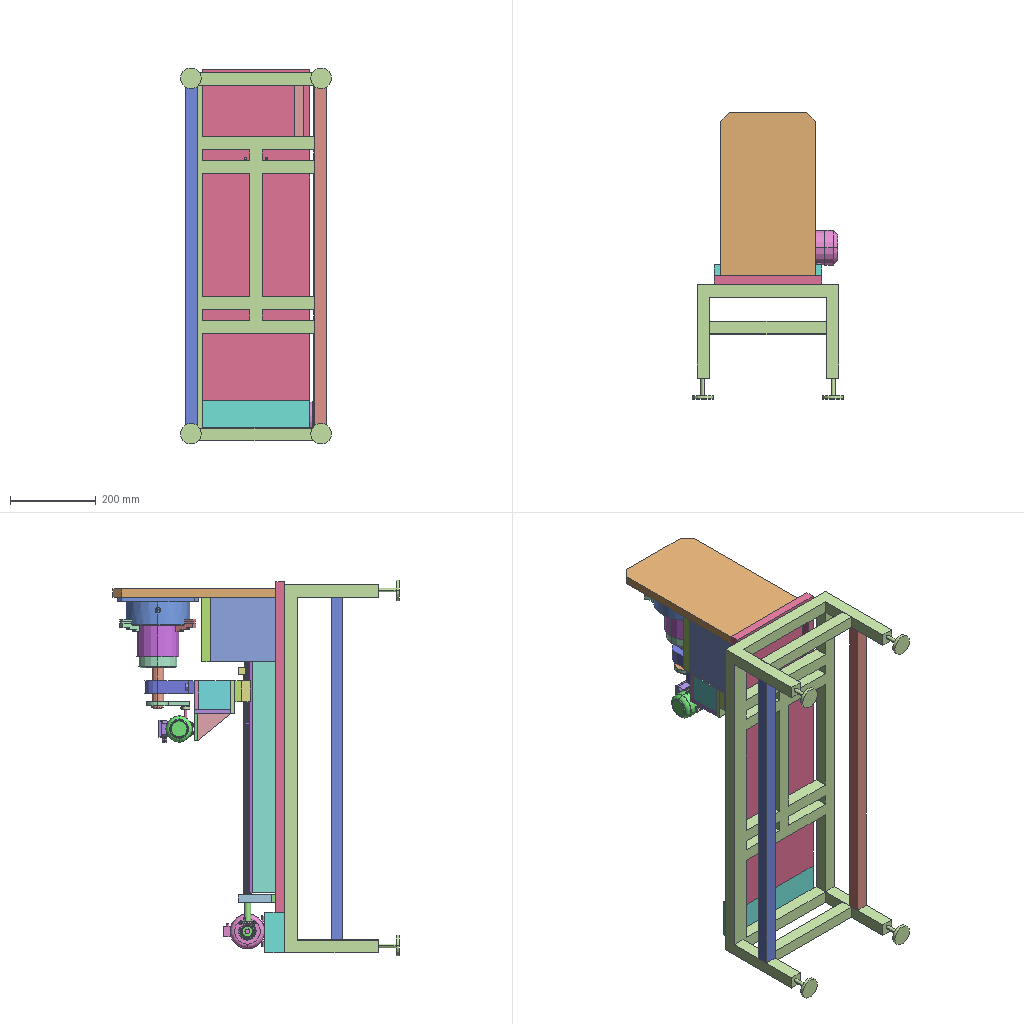Assembly | SolidWorks | 35 different items | 78 placed | box 352 x 667 x 876 mm
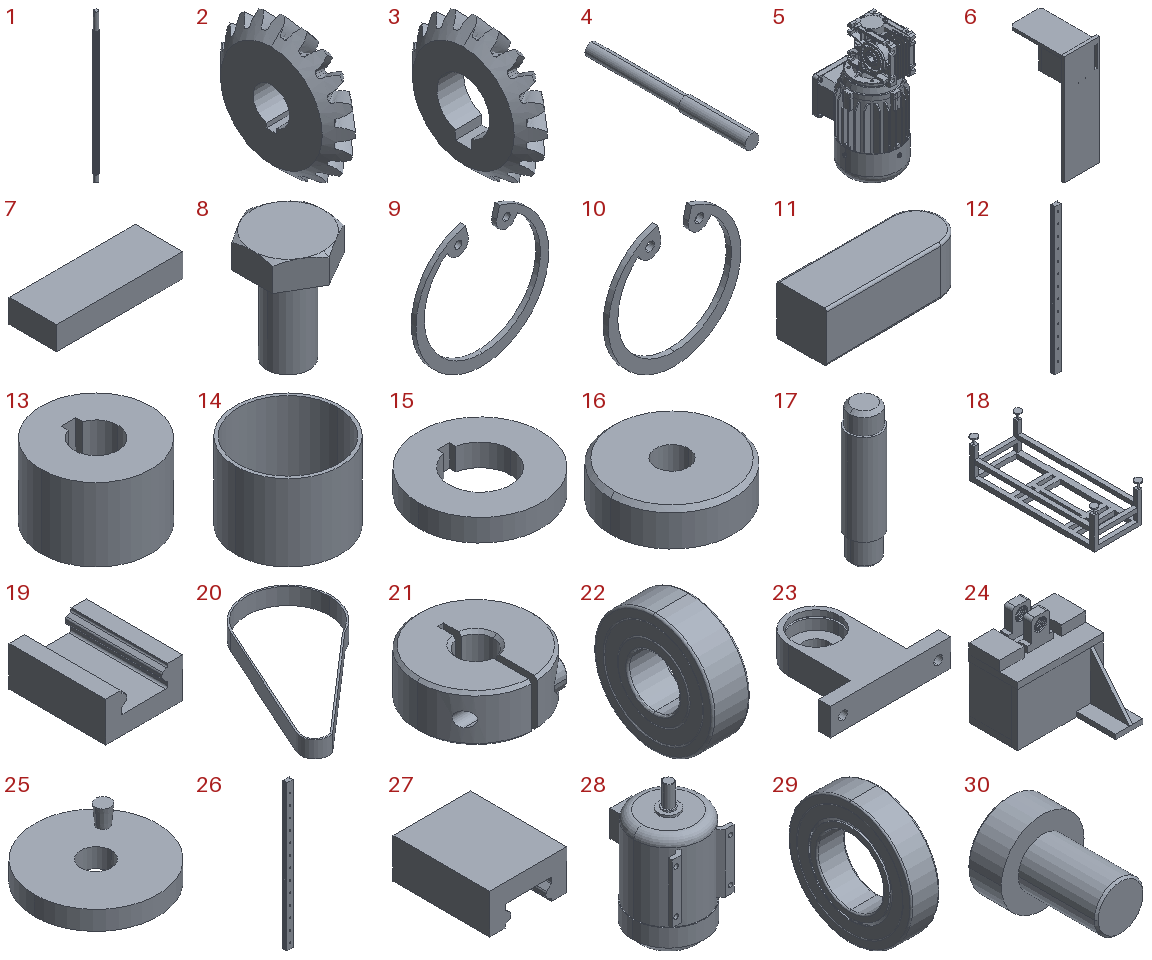Parts list (item | quantity | size | volume | features):
1 | x1 | 20 x 20 x 613.565 mm | 157929 mm3 | features MoveFace 3, Cut 2, ICE 2, Extrusion 1, SweepThread 1
2 | x1 | 10.311 x 40.668 x 40.791 mm | 6619 mm3 | features 3DProfileFeature 12, ICE 2, BlendCut 1, CirPattern 1, RefAxis 1, Revolution 1
3 | x1 | 10.311 x 40.668 x 40.791 mm | 5692 mm3 | features 3DProfileFeature 12, BlendCut 1, CirPattern 1, ICE 1, RefAxis 1, Revolution 1
4 | x1 | 7 x 80 x 7 mm | 2512 mm3 | features ICE 3, Extrusion 1
5 | x1 | 64.261 x 83.502 x 142.348 mm | 222279 mm3 | features BaseBody 11, Scale 1
6 | x1 | 250 x 399.718 x 770 mm | 8667321 mm3 | features ICE 10, MoveFace 8, HoleWzd 2, MirrorSolid 2, Chamfer 1, Cut 1, DelFace 1, Extrusion 1, MoveCopyBody 1
7 | x1 | 250 x 93.801 x 46.3 mm | 1085747 mm3 | features Extrusion 1, MoveFace 1
8 | x2 | 17 x 19.63 x 26.4 mm | 3167 mm3 | features ICE 1, MBimport 1
9 | x1 | 56.2 x 2 x 55.243 mm | 1250 mm3 | features Extrusion 1
10 | x2 | 37.8 x 1.5 x 37.156 mm | 475.123 mm3 | features Extrusion 1
11 | x1 | 14 x 5 x 5 mm | 331.224 mm3 | features Cut 1, Extrusion 1, Fillet 1
12 | x1 | 23.597 x 15.078 x 538 mm | 168139 mm3 | features Extrusion 1, HoleWzd 1
13 | x1 | 15 x 15 x 10 mm | 1468 mm3 | features Extrusion 1, ICE 1
14 | x1 | 98.909 x 98.909 x 72 mm | 65082 mm3 | features ExtruThin 1
15 | x1 | 50 x 50 x 9.018 mm | 13173 mm3 | features Extrusion 1, ICE 1, MoveFace 1
16 | x1 | 90.34 x 90.34 x 26 mm | 153646 mm3 | features Chamfer 1, Cut 1, Extrusion 1
17 | x1 | 28 x 28 x 118 mm | 66131 mm3 | features ICE 2, Chamfer 1, Cut 1, Extrusion 1, MoveFace 1
18 | x1 | 351.704 x 876.35 x 267 mm | 5919478 mm3 | features ICE 6, MirrorSolid 2, Extrusion 1, LPattern 1, MoveCopyBody 1, MoveFace 1, Split 1
19 | x1 | 38.915 x 48.81 x 20 mm | 27036 mm3 | features Cut 1, Extrusion 1
20 | x1 | 83.007 x 99.109 x 10 mm | 2707 mm3 | features ExtruThin 1
21 | x1 | 20 x 19.987 x 8 mm | 2133 mm3 | features BaseBody 2
22 | x2 | 11 x 35 x 35 mm | 6580 mm3 | features Revolution 5, CirPattern 2, RefAxis 1, RevCut 1
23 | x1 | 137.013 x 116.006 x 31 mm | 192152 mm3 | features ICE 3, Cut 1, Extrusion 1
24 | x1 | 137.013 x 140.341 x 138.543 mm | 535591 mm3 | features BaseBody 6, ICE 3, MoveCopyBody 2, SweepThread 2
25 | x1 | 64.655 x 64.655 x 20 mm | 31223 mm3 | features Extrusion 1, ICE 1
26 | x1 | 23.597 x 15.078 x 538 mm | 168139 mm3 | features MirrorStock 1
27 | x1 | 38.915 x 48.81 x 20 mm | 27036 mm3 | features MirrorStock 1
28 | x1 | 82 x 96 x 148.25 mm | 614858 mm3 | features Boss 9, Fillet 3, Chamfer 2, Attribute 1, Cut 1, Extrusion 1, LPattern 1, Scale 1
29 | x1 | 12 x 52 x 52 mm | 13563 mm3 | features Revolution 5, CirPattern 2, RefAxis 1, RevCut 1
30 | x32 | 8.5 x 11.5 x 8.5 mm | 331.771 mm3 | features Chamfer 1, ICE 1, MoveCopyBody 1, Revolution 1
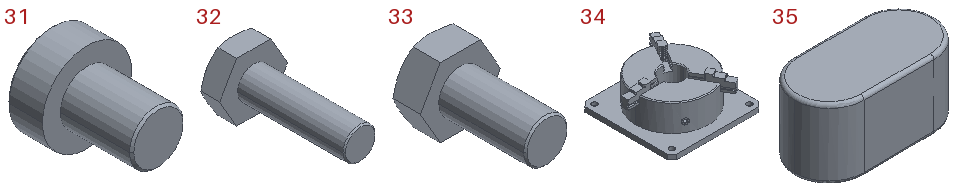31 | x4 | 10 x 12 x 10 mm | 492.529 mm3 | features Chamfer 1, ICE 1, MoveCopyBody 1, Revolution 1
32 | x4 | 6.351 x 12 x 5.5 mm | 122.833 mm3 | features ICE 2, Chamfer 1, DelFace 1, RevCut 1, Revolution 1
33 | x4 | 9.238 x 13.5 x 8 mm | 389.475 mm3 | features ICE 2, Chamfer 1, DelFace 1, RevCut 1, Revolution 1
34 | x1 | 193.6 x 190 x 79.5 mm | 1119464 mm3 | features BaseBody 4, MoveCopyBody 3, Chamfer 1, HoleWzd 1, ICE 1, MoveFace 1, Scale 1
35 | x1 | 10 x 5 x 4.997 mm | 220.26 mm3 | features Cut 1, Extrusion 1, Fillet 1
Mates (type | each side: item.copy, entity, surface, feature):
InPlace | 14.1 face plane Extrude-Thin1 | 16.1 plane
InPlace | 16.1 face plane Boss-Extrude1 | 17.1 plane
InPlace | 23.1 face plane Boss-Extrude1 | 24.1 plane
InPlace | 17.1 face plane Boss-Extrude2 | 15.1 plane
Coincident | 15.1 face plane Boss-Extrude1 | 13.1 face plane Boss-Extrude1
InPlace | 24.1 face plane Boss-Extrude9 | 19.1 plane
InPlace | 6.1 face plane Boss-Extrude2 | 12.1 plane
InPlace | 13.1 face plane Boss-Extrude1 | 20.1 plane
InPlace | 6.1 face plane Boss-Extrude4 | 18.1 plane
InPlace | 18.1 face plane Boss-Extrude1 | 7.1 plane
Concentric | 13.1 face cylinder Boss-Extrude1 | 5.1 face cylinder ML9A-1-solid1
Coincident | 24.1 face plane Boss-Extrude7 | 5.1 face plane E030-1-solid1
Concentric | 5.1 face cylinder ML9A-1-solid1 | 4.1 face cylinder Boss-Extrude1
Coincident | 5.1 face plane ML9A-1-solid1 | 4.1 face plane Cut-Extrude1
Coincident | 5.1 face plane ML9A-1-solid1 | 4.1 face plane Boss-Extrude1
Coincident | 13.1 face plane Boss-Extrude1 | 4.1 face plane Boss-Extrude2
Concentric | 5.1 face cylinder E030-1-solid1 | 32.1 face cylinder Revolve1
Coincident | 5.1 face plane E030-1-solid1 | 32.1 face plane Revolve1
Concentric | 5.1 face cylinder E030-1-solid1 | 32.2 face cylinder Revolve1
Coincident | 5.1 face plane E030-1-solid1 | 32.2 face plane Revolve1
Concentric | 5.1 face cylinder E030-1-solid1 | 32.3 face cylinder Revolve1
Coincident | 5.1 face plane E030-1-solid1 | 32.3 face plane Revolve1
Concentric | 5.1 face cylinder E030-1-solid1 | 32.4 face cylinder Revolve1
Coincident | 5.1 face plane E030-1-solid1 | 32.4 face plane Revolve1
Concentric | 28.1 edge | 33.1 face cylinder Revolve1
Coincident | 28.1 face plane Extrude9 | 33.1 face plane Revolve1
Concentric | 28.1 face cylinder LPattern1 | 33.2 face cylinder Revolve1
Coincident | 28.1 face plane Extrude9 | 33.2 face plane Revolve1
Concentric | 28.1 face cylinder Cut-Extrude1 | 33.3 face cylinder Revolve1
Coincident | 28.1 face plane Extrude9 | 33.3 face plane Revolve1
Concentric | 28.1 face cylinder LPattern1 | 33.4 face cylinder Revolve1
Coincident | 28.1 face plane Extrude9 | 33.4 face plane Revolve1
Concentric | 14.1 face cylinder Extrude-Thin1 | 34.1 face cylinder Chuck-1-solid1
Concentric | 4.1 face cylinder Boss-Extrude2 | 21.1 face cylinder STCB-D6-B8_base.stp-1-solid1
Coincident | 13.1 face plane Boss-Extrude1 | 21.1 face plane STCB-D6-B8_base.stp-1-solid1
Coincident | 6.1 face plane Boss-Extrude1 | 34.1 face plane Chuck-1-solid1
Parallel | 6.1 face plane Boss-Extrude1 | 34.1 face plane Boss-Extrude1
Concentric | 34.1 face cylinder CBORE for M6 Hexagon socket head cap screws1 | 31.1 face cylinder Revolve1
Coincident | 34.1 face plane CBORE for M6 Hexagon socket head cap screws1 | 31.1 face plane Revolve1
Concentric | 34.1 face cylinder CBORE for M6 Hexagon socket head cap screws1 | 31.2 face cylinder Revolve1
Coincident | 31.1 face plane Revolve1 | 31.2 face plane Revolve1
Concentric | 34.1 face cylinder CBORE for M6 Hexagon socket head cap screws1 | 31.3 face cylinder Revolve1
Coincident | 34.1 face plane CBORE for M6 Hexagon socket head cap screws1 | 31.3 face plane Revolve1
Concentric | 34.1 face cylinder CBORE for M6 Hexagon socket head cap screws1 | 31.4 face cylinder Revolve1
Coincident | 34.1 face plane CBORE for M6 Hexagon socket head cap screws1 | 31.4 face plane Revolve1
Concentric | 12.1 face cylinder CBORE for M5 Hexagon socket head cap screws1 | 30.1 face cylinder Revolve1
Coincident | 12.1 face plane CBORE for M5 Hexagon socket head cap screws1 | 30.1 face plane Revolve1
Concentric | 23.1 face cylinder Cut-Extrude1 | 8.1 face cylinder Hex Bolt SHBH SHBHS[SHBH-M10-L10].step<1>
Coincident | 23.1 face plane Boss-Extrude1 | 8.1 face plane Hex Bolt SHBH SHBHS[SHBH-M10-L10].step<1>
Concentric | 23.1 face cylinder Cut-Extrude1 | 8.2 face cylinder Hex Bolt SHBH SHBHS[SHBH-M10-L10].step<1>
Coincident | 23.1 face plane Boss-Extrude1 | 8.2 face plane Hex Bolt SHBH SHBHS[SHBH-M10-L10].step<1>
Concentric | 6.1 face cylinder CBORE for M5 Hexagon socket head cap screws2 | 30.2 face cylinder Revolve1
Coincident | 6.1 face plane CBORE for M5 Hexagon socket head cap screws2 | 30.2 edge
Concentric | 6.1 face cylinder CBORE for M5 Hexagon socket head cap screws2 | 30.3 face cylinder Revolve1
Coincident | 6.1 face plane CBORE for M5 Hexagon socket head cap screws2 | 30.3 face plane Revolve1
Concentric | 6.1 face cylinder CBORE for M5 Hexagon socket head cap screws1 | 30.4 face cylinder Revolve1
Coincident | 6.1 face plane CBORE for M5 Hexagon socket head cap screws1 | 30.4 face plane Revolve1
Concentric | 6.1 face cylinder CBORE for M5 Hexagon socket head cap screws1 | 30.5 face cylinder Revolve1
Coincident | 6.1 face plane CBORE for M5 Hexagon socket head cap screws1 | 30.5 face plane Revolve1
Parallel | 28.1 face plane Extrude8 | 7.1 face plane Boss-Extrude1
DistanceDim | 1.1 face plane Boss-Extrude1 | 6.1 face plane Boss-Extrude7
Concentric | 6.1 face cylinder Cut-Extrude2 | 1.1 face cylinder Cut-Extrude2
Parallel | 28.1 face plane Extrude9 | 7.1 face plane Boss-Extrude1
Coincident | 28.1 face plane Extrude4 | 2.1 face plane Revolve1
Concentric | 28.1 face cylinder Extrude4 | 2.1 face cylinder Cut-Extrude1
Concentric | 1.1 face cylinder Cut-Extrude2 | 3.1 face cylinder Cut-Extrude1
Coincident | 1.1 face plane Cut-Extrude4 | 3.1 face plane Cut-Extrude1
Concentric | 1.1 face cylinder Cut-Extrude4 | 11.1 face cylinder Extrude1
Coincident | 1.1 face plane Cut-Extrude4 | 11.1 face plane Extrude1
DistanceDim | 11.1 face plane Extrude1 | 1.1 face plane Cut-Extrude4
Coincident | 1.1 face plane Boss-Extrude1 | 3.1 face plane Revolve1
GearDim | 2.1 edge | 3.1 edge
Concentric | 17.1 face cylinder Boss-Extrude2 | 29.1 face cylinder Revolve1
Coincident | 23.1 face plane Cut-Extrude4 | 29.1 face plane Revolve1
Coincident | 29.1 face plane Revolve1 | 9.1 face plane Boss-Extrude1
Concentric | 23.1 face cylinder Boss-Extrude1 | 9.1 face cylinder Boss-Extrude1
Concentric | 6.1 face cylinder Cut-Extrude3 | 22.1 face cylinder Revolve1
Coincident | 6.1 face plane Cut-Extrude3 | 22.1 face plane Revolve1
Concentric | 6.1 face cylinder Cut-Extrude4 | 22.2 face cylinder Revolve1
Coincident | 6.1 face plane Cut-Extrude4 | 22.2 face plane Revolve1
Concentric | 6.1 face cylinder Cut-Extrude3 | 10.1 face cylinder Boss-Extrude1
Coincident | 22.1 face plane Revolve1 | 10.1 face plane Boss-Extrude1
Concentric | 6.1 face cylinder Cut-Extrude4 | 10.2 face cylinder Boss-Extrude1
Coincident | 22.2 face plane Revolve1 | 10.2 face plane Boss-Extrude1
Concentric | 17.1 face cylinder Cut-Extrude2 | 35.1 face cylinder Extrude1
Coincident | 17.1 face plane Cut-Extrude2 | 35.1 face plane Extrude1
Coincident | 15.1 face plane Cut-Extrude1 | 35.1 face plane Extrude1